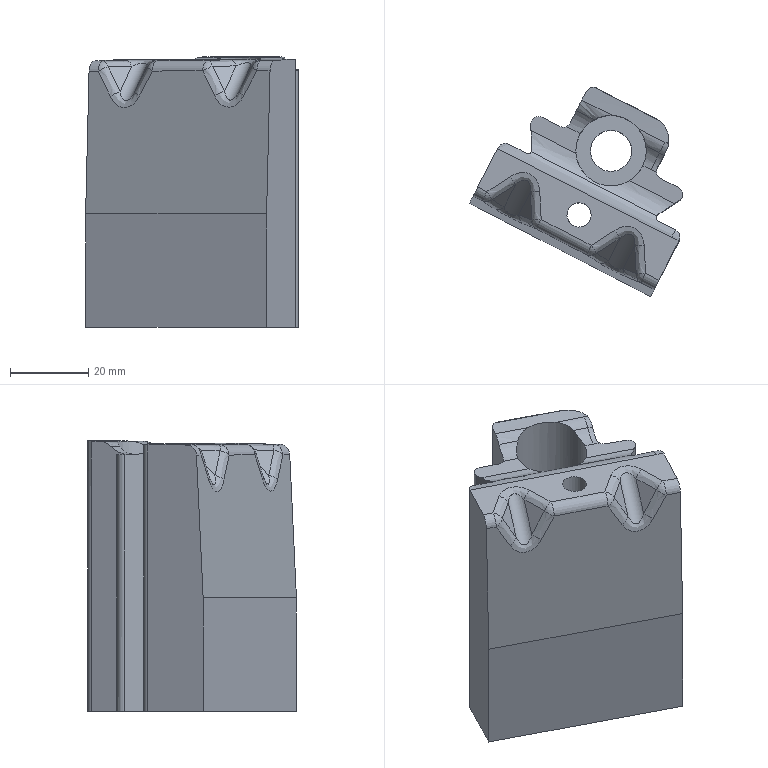Part | STEP file | gslz 2016.10.28-13_id30_x_t | 1 solid | 70 faces | box 54.348 x 53.334 x 69.186 mm | volume 92408 mm3 | spline 28 | cylinder 19 | plane 18 | sphere 4 | other 1 | commonest cylinder face diameters 4 x7 5.5 x5 2 x2 6.2 x1 10.3 x1 10.5 x1